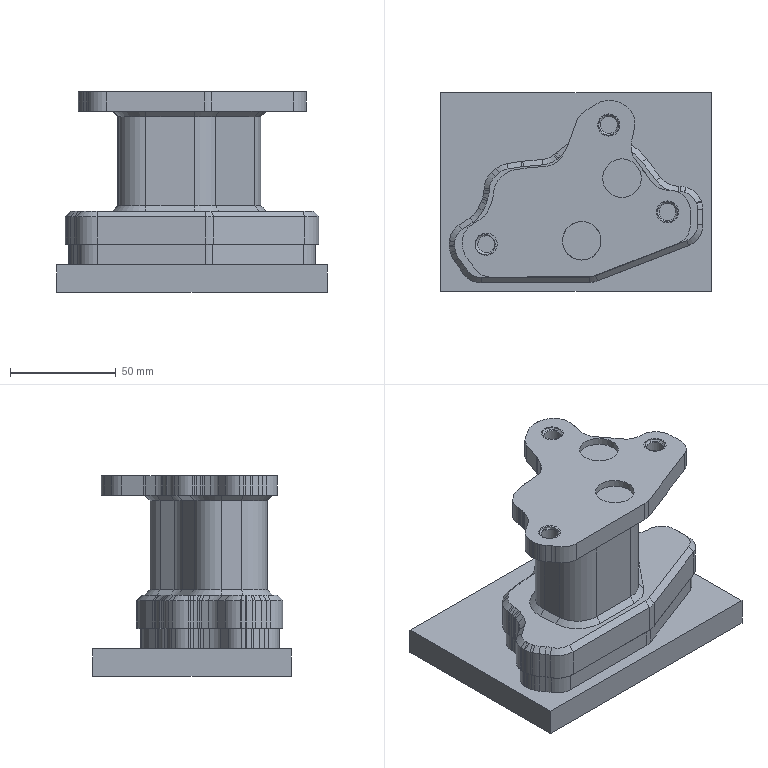NC program | NX | posted by the shop | part box 128.162 x 94.109 x 95 mm
Lines 6767 to 7617 of 131503:
6766 TOOL CALL 18 Z S7000
6767 CALL LBL101
6768 M3 M8
6769 M51
6770 CYCL DEF 32.0 TOLERANCE
6771 CYCL DEF 32.1 T0.012
6772 CYCL DEF 32.2 HSC-MODE:0
6773 L M126
6774 PLANE SPATIAL SPA-90. SPB+0.0 SPC-90. TURN FMAX SEQ-
6775 L X25.0162 Y76.3 FMAX
6776 L Z140. FMAX
6777 L Z60.952 FMAX
6778 L Z59.952 F3500.
6779 CC X23.3579 Y73.8
6780 C X23.3579 Y76.8 DR+
6781 L X20.2431
6782 CC X18.0112 Y72.1136
6783 C X23.2015 Y72.1821 DR-
6784 L Y59.1116
6785 CC X18.0193 Y59.1788
6786 C X19.1727 Y54.1262 DR-
6787 CC X15.4981 Y69.7463
6788 C X15.5573 Y53.6999 DR-
6789 L X8.3845
6790 CC X8.4524 Y69.8221
6791 C X4.7689 Y54.1262 DR-
6792 CC X5.9231 Y59.1793
6793 C X.7403 Y59.1116 DR-
6794 L Y72.1821
6795 CC X5.9307 Y72.1137
6796 C X3.6982 Y76.8 DR-
6797 L X.6876
6798 CC X.6876 Y73.8
6799 C X-.9707 Y76.3 DR+
6800 L Z60.952
6801 L X26.4232 Z60.4568 FMAX
6802 L Z59.4568
6803 CC X24.7649 Y73.8
6804 C X24.7649 Y76.8 DR+
6805 L X21.7693
6806 CC X19.5143 Y72.1369
6807 C X24.6939 Y72.1821 DR-
6808 L Y59.1096
6809 CC X19.5964 Y59.1096
6810 C X21.5012 Y54.3813 DR-
6811 CC X15.4288 Y69.4546
6812 C X15.5573 Y53.2047 DR-
6813 L X8.3845
6814 CC X8.5311 Y69.6316
6815 C X2.4459 Y54.3727 DR-
6816 CC X4.335 Y59.1096
6817 C X-.7648 Y59.1096 DR-
6818 L Y72.1822
6819 CC X4.3784 Y72.1579
6820 C X2.164 Y76.8 DR-
6821 L X-.9239
6822 CC X-.9239 Y73.8
6823 C X-2.5822 Y76.3 DR+
6824 L Z60.4568
6825 L Z140. FMAX
6826 L X27.488 FMAX
6827 L Z59.9615 FMAX
6828 L Z58.9615
6829 CC X25.8297 Y73.8
6830 C X25.8297 Y76.8 DR+
6831 L X22.8396
6832 CC X20.5081 Y72.129
6833 C X25.7284 Y72.1821 DR-
6834 L Y59.108
6835 CC X20.614 Y59.108
6836 C X22.8639 Y54.5152 DR-
6837 CC X14.6406 Y71.3021
6838 C X18.8893 Y53.0984 DR-
6839 CC X15.4932 Y67.7236
6840 C X15.5573 Y52.7095 DR-
6841 L X8.3845
6842 CC X8.4737 Y68.124
6843 C X3.7779 Y53.4419 DR-
6844 CC X11.4304 Y77.8698
6845 C X1.1148 Y54.4418 DR-
6846 CC X3.2768 Y59.1524
6847 C X-1.9061 Y59.1116 DR-
6848 L Y72.1822
6849 CC X3.3047 Y72.1316
6850 C X.9892 Y76.8 DR-
6851 L X-1.91
6852 CC X-1.91 Y73.8
6853 C X-3.5683 Y76.3 DR+
6854 L Z59.9615
6855 L Z140. FMAX
6856 L X28.2105 FMAX
6857 L Z59.4663 FMAX
6858 L Z58.4663
6859 CC X26.5522 Y73.8
6860 C X26.5522 Y76.8 DR+
6861 L X23.6689
6862 CC X21.3373 Y72.1408
6863 C X26.5472 Y72.1821 DR-
6864 L Y69.4374
6865 L X26.5601 Y69.1412 Z58.4789
6866 L X26.5962 Y68.8337 Z58.5141
6867 L X26.6521 Y68.5166 Z58.5685
6868 L X26.724 Y68.1917 Z58.6384
6869 L X27.0487 Y67.0211 Z58.9529
6870 L X27.3709 Y65.8509 Z59.2618
6871 L X27.4637 Y65.4084 Z59.3488
6872 L X27.5316 Y64.9754 Z59.411
6873 L X27.5744 Y64.549 Z59.4483
6874 L X27.592 Y64.1262 Z59.4607
6875 L X27.584 Y63.704 Z59.4483
6876 L X27.5503 Y63.2796 Z59.411
6877 L X27.4907 Y62.85 Z59.3488
6878 L X27.4049 Y62.4123 Z59.2618
6879 L X27.0904 Y61.258 Z58.9526
6880 L X26.7583 Y60.1058 Z58.6384
6881 L X26.6795 Y59.7849 Z58.5685
6882 L X26.6146 Y59.471 Z58.5141
6883 L X26.5669 Y59.1657 Z58.4789
6884 L X26.54 Y58.8706 Z58.4663
6885 CC X21.3606 Y59.1461
6886 C X24.1248 Y54.7574 DR-
6887 CC X13.5401 Y72.9332
6888 C X20.1486 Y52.9651 DR-
6889 CC X15.4311 Y67.399
6890 C X15.5573 Y52.2142 DR-
6891 L X8.3845
6892 CC X8.4544 Y66.9218
6893 C X4.1312 Y52.8638 DR-
6894 L X3.2815 Y53.1353
6895 L X2.7793 Y53.3142
6896 CC X11.0867 Y75.7801
6897 C X+0.0 Y54.5477 DR-
6898 CC X2.4105 Y59.1506
6899 C X-2.7852 Y59.1116 DR-
6900 L Y72.1822
6901 CC X2.4355 Y72.1343
6902 C X.0925 Y76.8 DR-
6903 L X-2.8569
6904 CC X-2.8569 Y73.8
6905 C X-4.5153 Y76.3 DR+
6906 L Z59.4663
6907 L Z140. FMAX
6908 L X28.9332 FMAX
6909 L Z58.9711 FMAX
6910 L Z57.9711
6911 CC X27.2749 Y73.8
6912 C X27.2749 Y76.8 DR+
6913 L X24.3788
6914 CC X21.9065 Y72.0368
6915 C X26.7613 Y74.324 DR-
6916 CC X22.3137 Y72.2287
6917 C X27.2301 Y72.2287 DR-
6918 L Y59.1082
6919 CC X22.1005 Y59.1082
6920 C X24.829 Y54.7644 DR-
6921 CC X11.97 Y75.2357
6922 C X21.1311 Y52.8638 DR-
6923 CC X15.3738 Y66.7537
6924 C X15.5573 Y51.719 DR-
6925 L X8.3845
6926 CC X8.5112 Y66.4939
6927 C X3.4322 Y52.6188 DR-
6928 L X2.9682 Y52.7842
6929 CC X10.9949 Y74.4406
6930 C X-1.0582 Y54.739 DR-
6931 CC X1.6163 Y59.1106
6932 C X-3.5085 Y59.1106 DR-
6933 L Y72.1822
6934 CC X1.6601 Y72.1657
6935 C X-1.3036 Y76.4002 DR-
6936 L X-1.2593 Y76.4302
6937 L X-.6675 Y76.8
6938 L X-3.5637
6939 CC X-3.5637 Y73.8
6940 C X-5.222 Y76.3 DR+
6941 L Z58.9711
6942 L Z140. FMAX
6943 L X7.0994 Y50.8734 FMAX
6944 L Z58.4759 FMAX
6945 L Z57.4759
6946 CC X5.1981 Y48.5529
6947 C X5.7128 Y51.5085 DR+
6948 CC X7.2984 Y60.613
6949 C X4.4075 Y51.8352 DR-
6950 L X3.7779 Y52.0349
6951 L X3.6592 Y52.0752
6952 L X3.157 Y52.2542
6953 CC X11.007 Y73.3789
6954 C X-.7066 Y54.1262 DR-
6955 CC X7.7287 Y68.7411
6956 C X-1.9308 Y54.9048 DR-
6957 CC X1.0054 Y59.1105
6958 C X-4.1239 Y59.1105 DR-
6959 L Y72.1822
6960 CC X1.0505 Y72.1684
6961 C X-1.9621 Y76.3754 DR-
6962 L X-1.8889 Y76.4257
6963 L X-1.3036 Y76.8
6964 L X-4.131
6965 CC X-4.131 Y73.8
6966 C X-5.7893 Y76.3 DR+
6967 L Z58.4759
6968 L Z140. FMAX
6969 L X5.387 Y50.8717 FMAX
6970 L Z57.9807 FMAX
6971 L Z56.9807
6972 CC X3.4454 Y48.5847
6973 C X4.0862 Y51.5155 DR+
6974 CC X5.4175 Y57.6042
6975 C X3.1482 Y51.7994 DR-
6976 CC X10.025 Y70.0458
6977 C X.6296 Y52.9593 DR-
6978 CC X15.3019 Y79.7897
6979 C X-2.5137 Y54.9351 DR-
6980 CC X.4788 Y59.1099
6981 C X-4.6577 Y59.1099 DR-
6982 L Y72.1853
6983 CC X.489 Y72.1853
6984 C X-2.3786 Y76.4591 DR-
6985 L X-1.8706 Y76.8
6986 L X-4.6713
6987 L X-4.9085 Y76.7832 Z56.9835
6988 L X-5.1227 Y76.7346 Z56.9915
6989 L X-5.3149 Y76.6568 Z57.0038
6990 L X-5.4862 Y76.5524 Z57.0196
6991 L X-5.6375 Y76.424 Z57.0382
6992 L X-5.7701 Y76.2743 Z57.0588
6993 L X-5.8848 Y76.1059 Z57.0804
6994 L X-5.9828 Y75.9215 Z57.1025
6995 L X-6.0651 Y75.7235 Z57.1241
6996 L X-6.1328 Y75.5148 Z57.1444
6997 L X-6.187 Y75.2978 Z57.1627
6998 L X-6.2286 Y75.0753 Z57.1782
6999 L X-6.2588 Y74.8499 Z57.1901
7000 L X-6.2857 Y74.4829 Z57.2001
7001 L X-6.2873 Y74.1196 Z57.1987
7002 L X-6.2657 Y73.7648 Z57.1861
7003 L X-6.2231 Y73.4229 Z57.1624
7004 L X-6.1616 Y73.0987 Z57.1281
7005 L X-6.0835 Y72.7967 Z57.0833
7006 L X-5.9908 Y72.5216 Z57.0282
7007 L X-5.8857 Y72.278 Z56.9631
7008 L X-5.821 Y72.1549 Z56.9216
7009 L X-5.754 Y72.0456 Z56.8778
7010 L X-5.6855 Y71.9521 Z56.8326
7011 L X-5.6166 Y71.8763 Z56.7867
7012 L X-5.5482 Y71.8203 Z56.7412
7013 L X-5.4812 Y71.786 Z56.6967
7014 L X-5.4167 Y71.7754 Z56.6543
7015 L X-5.3556 Y71.7906 Z56.6147
7016 L X-5.2989 Y71.8335 Z56.5788
7017 L X-5.2475 Y71.9061 Z56.5475
7018 L X-5.2024 Y72.0104 Z56.5216
7019 L X-5.1645 Y72.1483 Z56.5021
7020 L X-5.1349 Y72.322 Z56.4898
7021 L X-5.1145 Y72.5333 Z56.4855
7022 CC X.0126 Y72.1884
7023 C X-3.0261 Y76.3323 DR-
7024 L X-2.5659 Y76.6697
7025 L X-2.565 Y76.8
7026 L X-5.1158
7027 L X-5.3459 Y76.7848 Z56.4881
7028 L X-5.5548 Y76.7408 Z56.4954
7029 L X-5.7434 Y76.6701 Z56.5068
7030 L X-5.9127 Y76.5749 Z56.5216
7031 L X-6.0634 Y76.4575 Z56.5391
7032 L X-6.1966 Y76.32 Z56.5587
7033 L X-6.313 Y76.1646 Z56.5797
7034 L X-6.4138 Y75.9935 Z56.6014
7035 L X-6.4996 Y75.8089 Z56.6232
7036 L X-6.5715 Y75.613 Z56.6443
7037 L X-6.6303 Y75.4081 Z56.6642
7038 L X-6.677 Y75.1962 Z56.682
7039 L X-6.7125 Y74.9796 Z56.6973
7040 L X-6.7376 Y74.7606 Z56.7093
7041 L X-6.759 Y74.3767 Z56.7209
7042 L X-6.754 Y73.9967 Z56.7206
7043 L X-6.7249 Y73.6255 Z56.7087
7044 L X-6.6743 Y73.268 Z56.6853
7045 L X-6.6044 Y72.9292 Z56.6507
7046 L X-6.5178 Y72.6138 Z56.6052
7047 L X-6.4168 Y72.3268 Z56.549
7048 L X-6.3039 Y72.073 Z56.4823
7049 L X-6.2397 Y71.9531 Z56.4427
7050 L X-6.1737 Y71.8457 Z56.4008
7051 L X-6.1067 Y71.7524 Z56.3576
7052 L X-6.0396 Y71.6751 Z56.3136
7053 L X-5.9731 Y71.6152 Z56.2696
7054 L X-5.9083 Y71.5746 Z56.2264
7055 L X-5.8459 Y71.5548 Z56.1846
7056 L X-5.7868 Y71.5575 Z56.145
7057 L X-5.7318 Y71.5844 Z56.1083
7058 L X-5.6819 Y71.6372 Z56.0752
7059 L X-5.6378 Y71.7176 Z56.0466
7060 L X-5.6004 Y71.8271 Z56.023
7061 L X-5.5707 Y71.9676 Z56.0053
7062 L X-5.5493 Y72.1405 Z55.9941
7063 L X-5.5373 Y72.3477 Z55.9902
7064 CC X-.3833 Y72.1849
7065 C X-3.5685 Y76.2401 DR-
7066 L X-3.1558 Y76.5643
7067 L X-3.155 Y76.8
7068 L X-5.5381
7069 L X-5.7719 Y76.7846 Z55.9929
7070 L X-5.9837 Y76.7397 Z56.0004
7071 L X-6.1747 Y76.6677 Z56.0121
7072 L X-6.3456 Y76.5708 Z56.0272
7073 L X-6.4974 Y76.4512 Z56.0452
7074 L X-6.6311 Y76.3111 Z56.0652
7075 L X-6.7476 Y76.1528 Z56.0867
7076 L X-6.8478 Y75.9785 Z56.109
7077 L X-6.9328 Y75.7905 Z56.1313
7078 L X-7.0034 Y75.591 Z56.153
7079 L X-7.0605 Y75.3822 Z56.1734
7080 L X-7.1052 Y75.1664 Z56.1918
7081 L X-7.1384 Y74.9458 Z56.2076
7082 L X-7.161 Y74.7226 Z56.22
7083 L X-7.1775 Y74.3315 Z56.2323
7084 L X-7.1669 Y73.9444 Z56.2325
7085 L X-7.132 Y73.5663 Z56.2208
7086 L X-7.0752 Y73.2021 Z56.1975
7087 L X-6.9991 Y72.857 Z56.1628
7088 L X-6.9063 Y72.5359 Z56.1171
7089 L X-6.7993 Y72.2437 Z56.0604
7090 L X-6.6806 Y71.9855 Z55.993
7091 L X-6.6135 Y71.8636 Z55.953
7092 L X-6.5448 Y71.7545 Z55.9107
7093 L X-6.4752 Y71.6598 Z55.8669
7094 L X-6.4058 Y71.5813 Z55.8224
7095 L X-6.3374 Y71.5206 Z55.7779
7096 L X-6.2709 Y71.4795 Z55.7341
7097 L X-6.2072 Y71.4596 Z55.6918
7098 L X-6.1471 Y71.4626 Z55.6517
7099 L X-6.0917 Y71.4902 Z55.6146
7100 L X-6.0418 Y71.5441 Z55.5811
7101 L X-5.9983 Y71.626 Z55.5521
7102 L X-5.9621 Y71.7376 Z55.5282
7103 L X-5.934 Y71.8805 Z55.5103
7104 L X-5.9151 Y72.0565 Z55.499
7105 L X-5.9061 Y72.2673 Z55.495
7106 CC X-.7533 Y72.1842
7107 C X-4.1598 Y76.0513 DR-
7108 CC X2.1983 Y68.8335
7109 C X-3.6558 Y76.4657 DR-
7110 L Y76.8
7111 L X-5.9072
7112 CC X-5.9072 Y73.8
7113 C X-7.5656 Y76.3 DR+
7114 L Z56.495
7115 L Z140. FMAX
7116 L X4.1977 Y50.8722 FMAX
7117 L Z57.4855 FMAX
7118 L Z56.4855
7119 CC X2.2183 Y48.6178
7120 C X2.9239 Y51.5337 DR+
7121 CC X4.2828 Y57.1491
7122 C X1.8323 Y51.917 DR-
7123 CC X10.9093 Y70.8375
7124 C X+0.0 Y52.9109 DR-
7125 CC X18.0902 Y82.7941
7126 C X-2.7473 Y54.7574 DR-
7127 L X-3.0151 Y54.9525
7128 CC X.0108 Y59.1036
7129 C X-5.1103 Y58.7019 DR-
7130 L X-5.2212 Y58.972 Z56.5834
7131 L X-5.3137 Y59.2088 Z56.6821
7132 L X-5.3883 Y59.4134 Z56.7814
7133 L X-5.4453 Y59.5869 Z56.8809
7134 L X-5.4851 Y59.7304 Z56.9804
7135 L X-5.5083 Y59.845 Z57.0796
7136 L X-5.5153 Y59.9317 Z57.1782
7137 L X-5.5064 Y59.9917 Z57.276
7138 L X-5.4822 Y60.0259 Z57.3727
7139 L X-5.443 Y60.0355 Z57.4679
7140 L X-5.3893 Y60.0215 Z57.5615
7141 L X-5.3216 Y59.9851 Z57.6532
7142 L X-5.2402 Y59.9272 Z57.7426
7143 L X-5.1455 Y59.849 Z57.8295
7144 L X-5.0381 Y59.7516 Z57.9137
7145 L X-4.9184 Y59.636 Z57.9948
7146 L X-4.7867 Y59.5033 Z58.0726
7147 L X-4.6436 Y59.3545 Z58.1468
7148 L X-4.4894 Y59.1909 Z58.2171
7149 L X-4.2324 Y58.913 Z58.3158
7150 L X-4.0529 Y58.7171 Z58.375
7151 L X-3.8399 Y58.4839 Z58.4357
7152 L X-3.3813 Y57.9816 Z58.5345
7153 L X-2.6961 Y57.2332 Z58.6278
7154 L X-2.0904 Y56.5742 Z58.6699
7155 L X-1.6884 Y56.1383 Z58.6806
7156 L X-1.2863 Y55.7035 Z58.6776
7157 L X-.8341 Y55.2164 Z58.6583
7158 L X-.035 Y54.3609 Z58.5864
7159 L X.7208 Y53.5603 Z58.4654
7160 L X1.2877 Y52.9676 Z58.3328
7161 L X1.709 Y52.5339 Z58.202
7162 L X1.9307 Y52.3081 Z58.1204
7163 L X2.1178 Y52.1185 Z58.0431
7164 L X2.3845 Y51.8492 Z57.9172
7165 L X2.5429 Y51.6891 Z57.8296
7166 L X2.6878 Y51.5419 Z57.7386
7167 L X2.8182 Y51.4081 Z57.6446
7168 L X2.933 Y51.2883 Z57.5478
7169 L X3.031 Y51.183 Z57.4487
7170 L X3.1114 Y51.0929 Z57.3474
7171 L X3.173 Y51.0184 Z57.2444
7172 L X3.2148 Y50.9601 Z57.14
7173 L X3.2357 Y50.9185 Z57.0345
7174 L X3.2346 Y50.8943 Z56.9282
7175 L X3.2105 Y50.8879 Z56.8214
7176 L X3.1624 Y50.8999 Z56.7145
7177 L X3.0892 Y50.9309 Z56.6078
7178 L X2.9898 Y50.9814 Z56.5017
7179 L X2.8632 Y51.052 Z56.3964
7180 L X2.7083 Y51.1432 Z56.2923
7181 L X2.5241 Y51.2556 Z56.1897
7182 L X2.3095 Y51.3897 Z56.0889
7183 L X2.0635 Y51.5461 Z55.9902
7184 CC X3.4481 Y56.9528
7185 C X.6296 Y52.1355 DR-
7186 CC X20.9038 Y85.7486
7187 C X-3.6072 Y55.0877 DR-
7188 CC X-.394 Y59.1071
7189 C X-5.535 Y58.8829 DR-
7190 CC X-8.5321 Y58.7522
7191 C X-6.0399 Y60.4222 DR+
7192 L Z56.9902
7193 L Z64.9328 FMAX
7194 L X2.547 Y50.8759 FMAX
7195 L Z56.495 FMAX
7196 L Z55.495
7197 CC X.4951 Y48.6874
7198 C X1.3117 Y51.5741 DR+
7199 CC X2.7712 Y56.7335
7200 C X-.1428 Y52.2326 DR-
7201 CC X25.9131 Y91.2207
7202 C X-4.0529 Y55.1511 DR-
7203 CC X-.7293 Y59.1209
7204 C X-5.9027 Y58.9147 DR-
7205 CC X-8.9003 Y58.7953
7206 C X-6.4068 Y60.4633 DR+
7207 L Z56.495
7208 L Z64.9328 FMAX
7209 L X1.9373 Y50.8805 FMAX
7210 L Z55.9998 FMAX
7211 L Z54.9998
7212 CC X-.1472 Y48.723
7213 C X.7093 Y51.5981 DR+
7214 CC X2.2636 Y56.8156
7215 C X-.6748 Y52.2326 DR-
7216 CC X29.4269 Y94.2142
7217 C X-4.193 Y54.9934 DR-
7218 L X-4.4075 Y55.1704
7219 CC X-1.0324 Y59.1262
7220 C X-6.2323 Y59.1116 DR-
7221 L Y72.1841
7222 CC X-1.0763 Y72.1841
7223 C X-4.4868 Y76.0511 DR-
7224 CC X4.4092 Y65.9644
7225 C X-4.0864 Y76.3906 DR-
7226 L Y76.8
7227 L X-6.2526
7228 CC X-6.2526 Y73.8
7229 C X-7.911 Y76.3 DR+
7230 L Z55.9998
7231 L Z140. FMAX
7232 L X1.3858 Y50.8863 FMAX
7233 L Z55.5046 FMAX
7234 L Z54.5046
7235 CC X-.7355 Y48.765
7236 C X.173 Y51.6241 DR+
7237 CC X1.8013 Y56.7479
7238 C X-1.1171 Y52.2326 DR-
7239 CC X25.2759 Y87.6031
7240 C X-3.7779 Y54.3835 DR-
7241 CC X11.6418 Y73.3652
7242 C X-4.9386 Y55.3885 DR-
7243 CC X-1.3091 Y59.1289
7244 C X-6.5209 Y59.1116 DR-
7245 L Y72.1822
7246 CC X-1.2815 Y72.1576
7247 C X-4.5933 Y76.2176 DR-
7248 L X-4.4698 Y76.3215
7249 L X-4.459 Y76.3435
7250 L Y76.8
7251 L X-6.5458
7252 L X-6.7791 Y76.7834 Z54.5074
7253 L X-6.9889 Y76.7355 Z54.5152
7254 L X-7.1763 Y76.6588 Z54.5272
7255 L X-7.3424 Y76.5559 Z54.5427
7256 L X-7.4882 Y76.4293 Z54.5609
7257 L X-7.615 Y76.2817 Z54.581
7258 L X-7.7236 Y76.1157 Z54.6022
7259 L X-7.8154 Y75.9339 Z54.6237
7260 L X-7.8913 Y75.7388 Z54.6448
7261 L X-7.9524 Y75.533 Z54.6646
7262 L X-7.9999 Y75.3191 Z54.6824
7263 L X-8.0348 Y75.0997 Z54.6974
7264 L X-8.0582 Y74.8774 Z54.7088
7265 L X-8.0741 Y74.5155 Z54.7183
7266 L X-8.0648 Y74.1573 Z54.7165
7267 L X-8.0324 Y73.8074 Z54.7036
7268 L X-7.979 Y73.4701 Z54.68
7269 L X-7.9068 Y73.1501 Z54.6457
7270 L X-7.8181 Y72.8519 Z54.6011
7271 L X-7.7148 Y72.58 Z54.5464
7272 L X-7.5993 Y72.339 Z54.4819
7273 L X-7.5287 Y72.217 Z54.4408
7274 L X-7.4558 Y72.1086 Z54.3974
7275 L X-7.3815 Y72.0156 Z54.3527
7276 L X-7.3069 Y71.9402 Z54.3073
7277 L X-7.2329 Y71.8841 Z54.2622
7278 L X-7.1605 Y71.8495 Z54.2182
7279 L X-7.0907 Y71.8383 Z54.1762
7280 L X-7.0244 Y71.8524 Z54.1371
7281 L X-6.9627 Y71.8939 Z54.1016
7282 L X-6.9065 Y71.9647 Z54.0707
7283 L X-6.8568 Y72.0668 Z54.0451
7284 L X-6.8147 Y72.2022 Z54.0258
7285 L X-6.7809 Y72.3728 Z54.0136
7286 L X-6.7567 Y72.5806 Z54.0094
7287 CC X-1.3275 Y72.1213
7288 C X-6.3109 Y74.324 DR-
7289 CC X-1.5296 Y72.1327
7290 C X-4.8956 Y76.1741 DR-
7291 L X-4.8435 Y76.2176
7292 L X-4.7822 Y76.2765
7293 L Y76.8
7294 L X-6.7581
7295 L X-6.9929 Y76.7833 Z54.0122
7296 L X-7.2039 Y76.7351 Z54.0201
7297 L X-7.3924 Y76.6578 Z54.0322
7298 L X-7.5595 Y76.5542 Z54.0479
7299 L X-7.7061 Y76.4267 Z54.0662
7300 L X-7.8335 Y76.2781 Z54.0865
7301 L X-7.9428 Y76.1109 Z54.1079
7302 L X-8.035 Y75.9278 Z54.1296
7303 L X-8.1112 Y75.7313 Z54.1509
7304 L X-8.1725 Y75.524 Z54.1709
7305 L X-8.2201 Y75.3086 Z54.189
7306 L X-8.255 Y75.0877 Z54.2042
7307 L X-8.2784 Y74.8638 Z54.2158
7308 L X-8.2941 Y74.4994 Z54.2255
7309 L X-8.2844 Y74.1387 Z54.2238
7310 L X-8.2515 Y73.7862 Z54.211
7311 L X-8.1977 Y73.4466 Z54.1874
7312 L X-8.125 Y73.1244 Z54.1531
7313 L X-8.0358 Y72.8243 Z54.1084
7314 L X-7.9322 Y72.5507 Z54.0535
7315 L X-7.8165 Y72.3082 Z53.9888
7316 L X-7.7458 Y72.1856 Z53.9475
7317 L X-7.6729 Y72.0767 Z53.904
7318 L X-7.5988 Y71.9833 Z53.859
7319 L X-7.5244 Y71.9076 Z53.8135
7320 L X-7.4507 Y71.8515 Z53.7682
7321 L X-7.3787 Y71.8169 Z53.724
7322 L X-7.3095 Y71.8059 Z53.6818
7323 L X-7.244 Y71.8204 Z53.6425
7324 L X-7.1832 Y71.8624 Z53.6069
7325 L X-7.1282 Y71.9339 Z53.5758
7326 L X-7.0798 Y72.0369 Z53.5501
7327 L X-7.0391 Y72.1734 Z53.5307
7328 L X-7.0071 Y72.3452 Z53.5184
7329 L X-6.9848 Y72.5545 Z53.5142
7330 CC X-1.7586 Y72.1635
7331 C X-5.0798 Y76.2176 DR-
7332 L X-5.0617 Y76.2433
7333 L Y76.8
7334 L X-6.9863
7335 L X-7.2165 Y76.7837 Z53.5169
7336 L X-7.4234 Y76.7364 Z53.5245
7337 L X-7.6082 Y76.6607 Z53.5364
7338 L X-7.772 Y76.5592 Z53.5516
7339 L X-7.9157 Y76.4344 Z53.5694
7340 L X-8.0406 Y76.2889 Z53.5891
7341 L X-8.1476 Y76.1251 Z53.6099
7342 L X-8.2379 Y75.9458 Z53.6309
7343 L X-8.3126 Y75.7533 Z53.6515
7344 L X-8.3726 Y75.5504 Z53.6709
7345 L X-8.4192 Y75.3394 Z53.6883
7346 L X-8.4533 Y75.1231 Z53.7029
7347 L X-8.4761 Y74.9039 Z53.7139
7348 L X-8.4913 Y74.547 Z53.7229
7349 L X-8.4816 Y74.1937 Z53.7208
7350 L X-8.4489 Y73.8486 Z53.7077
7351 L X-8.3956 Y73.516 Z53.6839
7352 L X-8.3237 Y73.2003 Z53.6497
7353 L X-8.2353 Y72.9061 Z53.6053
7354 L X-8.1325 Y72.6379 Z53.551
7355 L X-8.0175 Y72.3999 Z53.487
7356 L X-7.9472 Y72.2795 Z53.4462
7357 L X-7.8746 Y72.1724 Z53.4032
7358 L X-7.8006 Y72.0806 Z53.3589
7359 L X-7.7262 Y72.006 Z53.3139
7360 L X-7.6523 Y71.9505 Z53.2693
7361 L X-7.58 Y71.9162 Z53.2257
7362 L X-7.5102 Y71.905 Z53.1841
7363 L X-7.4438 Y71.9188 Z53.1454
7364 L X-7.3819 Y71.9595 Z53.1103
7365 L X-7.3254 Y72.0292 Z53.0796
7366 L X-7.2752 Y72.1298 Z53.0543
7367 L X-7.2324 Y72.2632 Z53.0352
7368 L X-7.1979 Y72.4314 Z53.0232
7369 L X-7.1726 Y72.6363 Z53.0189
7370 CC X-1.9439 Y72.162
7371 C X-5.3041 Y76.1959 DR-
7372 L X-5.3022 Y76.2063
7373 L Y76.8
7374 L X-7.1733
7375 L X-7.4077 Y76.7833 Z53.0217
7376 L X-7.6182 Y76.7351 Z53.0296
7377 L X-7.8059 Y76.6579 Z53.0417
7378 L X-7.972 Y76.5543 Z53.0574
7379 L X-8.1175 Y76.4269 Z53.0757
7380 L X-8.2437 Y76.2784 Z53.0959
7381 L X-8.3515 Y76.1113 Z53.1173
7382 L X-8.4421 Y75.9282 Z53.139
7383 L X-8.5167 Y75.7318 Z53.1603
7384 L X-8.5763 Y75.5247 Z53.1803
7385 L X-8.6221 Y75.3094 Z53.1982
7386 L X-8.6552 Y75.0885 Z53.2134
7387 L X-8.6766 Y74.8648 Z53.225
7388 L X-8.6892 Y74.5005 Z53.2347
7389 L X-8.6763 Y74.1399 Z53.233
7390 L X-8.6401 Y73.7876 Z53.2202
7391 L X-8.583 Y73.4482 Z53.1965
7392 L X-8.5072 Y73.1261 Z53.1622
7393 L X-8.4149 Y72.8261 Z53.1176
7394 L X-8.3083 Y72.5527 Z53.0627
7395 L X-8.1897 Y72.3103 Z52.998
7396 L X-8.1175 Y72.1878 Z52.9568
7397 L X-8.0431 Y72.0789 Z52.9133
7398 L X-7.9676 Y71.9857 Z52.8683
7399 L X-7.8919 Y71.91 Z52.8228
7400 L X-7.817 Y71.8539 Z52.7775
7401 L X-7.744 Y71.8194 Z52.7334
7402 L X-7.6738 Y71.8084 Z52.6913
7403 L X-7.6076 Y71.8229 Z52.652
7404 L X-7.5462 Y71.8649 Z52.6163
7405 L X-7.4906 Y71.9363 Z52.5853
7406 L X-7.442 Y72.0393 Z52.5596
7407 L X-7.4013 Y72.1756 Z52.5403
7408 L X-7.3695 Y72.3473 Z52.528
7409 L X-7.3476 Y72.5564 Z52.5237
7410 CC X-2.1887 Y72.1821
7411 C X-5.7554 Y75.9282 DR-
7412 L X-5.5069 Y76.1648
7413 L Y76.8
7414 L X-7.3476
7415 CC X-7.3476 Y73.8
7416 C X-9.006 Y76.3 DR+
7417 L Z53.5237
7418 L Z140. FMAX
7419 L X.9138 Y50.8926 FMAX
7420 L Z55.0094 FMAX
7421 L Z54.0094
7422 CC X-1.2416 Y48.8058
7423 C X-.2832 Y51.6486 DR+
7424 CC X1.4056 Y56.6582
7425 C X-1.9194 Y52.5482 DR-
7426 CC X73.6911 Y143.344
7427 C X-5.0371 Y55.2379 DR-
7428 CC X-1.541 Y59.134
7429 C X-6.7516 Y58.6318 DR-
7430 CC X-9.7378 Y58.3439
7431 C X-7.2757 Y60.0581 DR+
7432 L Z55.0094
7433 L Z63.9424 FMAX
7434 L X-.6846 Y51.1486 FMAX
7435 L Z54.5142 FMAX
7436 L Z53.5142
7437 CC X-3.6412 Y51.6574
7438 C X-.6412 Y51.6611 DR+
7439 CC X1.0818 Y56.6434
7440 C X-2.238 Y52.5482 DR-
7441 CC X72.7011 Y139.7779
7442 C X-5.4227 Y55.3885 DR-
7443 CC X-1.7936 Y59.1209
7444 C X-6.98 Y58.6721 DR-
7445 CC X-9.9689 Y58.4135
7446 C X-7.4994 Y60.1169 DR+
7447 L Z54.5142
7448 L Z140. FMAX
7449 L X29.5035 Y76.3 FMAX
7450 L Z58.4759 FMAX
7451 L Z57.4759
7452 CC X27.8452 Y73.8
7453 C X27.8452 Y76.8 DR+
7454 L X25.0106
7455 L X25.5215 Y76.4701
7456 CC X22.6292 Y72.1649
7457 C X27.8157 Y72.1821 DR-
7458 L Y59.109
7459 CC X22.6875 Y59.109
7460 C X25.5985 Y54.8871 DR-
7461 CC X10.2489 Y77.1492
7462 C X22.0375 Y52.8132 DR-
7463 CC X14.6615 Y68.0151
7464 C X18.6733 Y51.6014 DR-
7465 CC X16.6458 Y60.4197
7466 C X18.2309 Y51.5113 DR-
7467 CC X18.7564 Y48.5577
7468 C X16.8494 Y50.8735 DR+
7469 L Z58.4759
7470 L Z65.9233 FMAX
7471 L X28.8259 Y60.2667 FMAX
7472 L Z57.9807 FMAX
7473 L Z56.9807
7474 CC X31.3089 Y58.583
7475 C X28.3152 Y58.7768 DR+
7476 CC X23.1855 Y59.1089
7477 C X26.2032 Y54.9476 DR-
7478 CC X5.9809 Y82.8343
7479 C X23.2968 Y53.0556 DR-
7480 CC X12.4366 Y71.8273
7481 C X20.7782 Y51.8088 DR-
7482 CC X18.4878 Y57.5894
7483 C X19.8024 Y51.5122 DR-
7484 L X19.5517 Y51.3652 Z57.0786
7485 L X19.3354 Y51.2395 Z57.1774
7486 L X19.1521 Y51.1344 Z57.2766
7487 L X19.0009 Y51.0496 Z57.3761
7488 L X18.8806 Y50.9844 Z57.4756
7489 L X18.79 Y50.9383 Z57.5748
7490 L X18.7279 Y50.9109 Z57.6735
7491 L X18.6933 Y50.9015 Z57.7712
7492 L X18.6849 Y50.9098 Z57.8679
7493 L X18.7015 Y50.9351 Z57.9632
7494 L X18.7422 Y50.977 Z58.0567
7495 L X18.8056 Y51.035 Z58.1484
7496 L X18.8907 Y51.1084 Z58.2378
7497 L X18.9962 Y51.1969 Z58.3247
7498 L X19.1211 Y51.2998 Z58.4089
7499 L X19.2641 Y51.4167 Z58.49
7500 L X19.4242 Y51.5471 Z58.5678
7501 L X19.6002 Y51.6903 Z58.642
7502 L X19.8989 Y51.9347 Z58.7474
7503 L X20.356 Y52.3133 Z58.8742
7504 L X21.0061 Y52.8647 Z59.0023
7505 L X21.416 Y53.2183 Z59.0623
7506 L X21.8188 Y53.5695 Z59.1076
7507 L X22.2467 Y53.9459 Z59.1425
7508 L X22.6943 Y54.3427 Z59.1655
7509 L X23.1545 Y54.7533 Z59.1758
7510 L X23.6215 Y55.1721 Z59.1728
7511 L X24.0899 Y55.594 Z59.1566
7512 L X24.5551 Y56.0144 Z59.1272
7513 L X25.012 Y56.4281 Z59.0848
7514 L X25.4547 Y56.8294 Z59.0302
7515 L X25.8863 Y57.2208 Z58.963
7516 L X26.516 Y57.7915 Z58.8384
7517 L X27.1716 Y58.3836 Z58.6654
7518 L X27.5406 Y58.7134 Z58.5382
7519 L X27.8485 Y58.984 Z58.4124
7520 L X28.0348 Y59.1436 Z58.3248
7521 L X28.2087 Y59.2888 Z58.2338
7522 L X28.3697 Y59.4183 Z58.1398
7523 L X28.5172 Y59.5311 Z58.043
7524 L X28.6508 Y59.6262 Z57.9439
7525 L X28.7697 Y59.7025 Z57.8426
7526 L X28.8735 Y59.7589 Z57.7396
7527 L X28.9616 Y59.7943 Z57.6352
7528 L X29.0335 Y59.8077 Z57.5297
7529 L X29.0886 Y59.7981 Z57.4234
7530 L X29.1264 Y59.7643 Z57.3166
7531 L X29.1463 Y59.7053 Z57.2097
7532 L X29.1478 Y59.6201 Z57.1031
7533 L X29.1303 Y59.5075 Z56.9969
7534 L X29.0932 Y59.3665 Z56.8916
7535 L X29.036 Y59.1961 Z56.7875
7536 L X28.9582 Y58.9951 Z56.6849
7537 L X28.8592 Y58.7626 Z56.5841
7538 L X28.7385 Y58.4974 Z56.4855
7539 CC X23.6211 Y59.1085
7540 C X26.7578 Y55.0192 DR-
7541 CC X3.844 Y84.8922
7542 C X22.6671 Y52.2865 DR-
7543 CC X18.7333 Y59.0055
7544 C X21.4078 Y51.6934 DR-
7545 CC X19.5481 Y56.9066
7546 C X20.8463 Y51.526 DR-
7547 CC X21.5499 Y48.6097
7548 C X19.5793 Y50.8717 DR+
7549 L Z57.4855
7550 L Z65.428 FMAX
7551 L X29.6721 Y60.5242 FMAX
7552 L Z56.9902 FMAX
7553 L Z55.9902
7554 CC X32.1684 Y58.8603
7555 C X29.1697 Y58.9509 DR+
7556 CC X24.0284 Y59.1062
7557 C X27.2324 Y55.0822 DR-
7558 CC X-8.2323 Y99.6229
7559 C X25.1857 Y53.5268 DR-
7560 CC X5.1203 Y81.3898
7561 C X23.2539 Y52.2326 DR-
7562 CC X20.2899 Y56.9035
7563 C X21.6653 Y51.5453 DR-
7564 CC X22.4112 Y48.6395
7565 C X20.4081 Y50.8727 DR+
7566 L Z56.9902
7567 L Z63.9424 FMAX
7568 L X23.8816 Y37.3963 FMAX
7569 L Z55.0094 FMAX
7570 L Z54.0094
7571 CC X23.5647 Y34.4131
7572 C X23.3816 Y37.4075 DR+
7573 CC X22.2041 Y56.6687
7574 C X22.24 Y37.3716 DR-
7575 L X1.6163
7576 L X1.6145 Y43.4182
7577 L X1.6015 Y43.4847
7578 L X1.5258 Y44.0788
7579 L X1.5248 Y44.3716
7580 L X22.2321
7581 CC X22.2041 Y56.6687
7582 C X23.561 Y44.4467 DR+
7583 L X23.5671 Y51.5499
7584 CC X22.2042 Y56.6687
7585 C X22.221 Y51.3716 DR-
7586 L X1.5008
7587 CC X1.5008 Y48.3716
7588 C X.0952 Y51.022 DR+
7589 L Z55.0094
7590 L X1.1191 Y27.5841 FMAX
7591 L Z54.0094
7592 CC X.7912 Y30.5662
7593 C X1.6191 Y27.6827 DR+
7594 CC X6.9063 Y9.2686
7595 C X1.9978 Y27.7872 DR-
7596 CC X7.0085 Y9.7522
7597 C X3.9703 Y28.2221 DR-
7598 CC X7.6309 Y5.9689
7599 C X7.6927 Y28.5211 DR-
7600 L X17.2822
7601 CC X17.4736 Y6.9113
7602 C X23.3092 Y27.7191 DR-
7603 CC X18.1055 Y9.2572
7604 C X23.3788 Y27.6994 DR-
7605 L X23.3766 Y20.2389
7606 CC X18.1054 Y9.2572
7607 C X21.4144 Y20.9804 DR+
7608 CC X17.4736 Y6.9113
7609 C X17.3162 Y21.5211 DR+
7610 L X7.6822
7611 CC X7.6309 Y5.9689
7612 C X5.1065 Y21.315 DR+
7613 CC X7.0085 Y9.7522
7614 C X3.8317 Y21.0315 DR+
7615 CC X6.9063 Y9.2686
7616 C X1.6213 Y20.2179 DR+